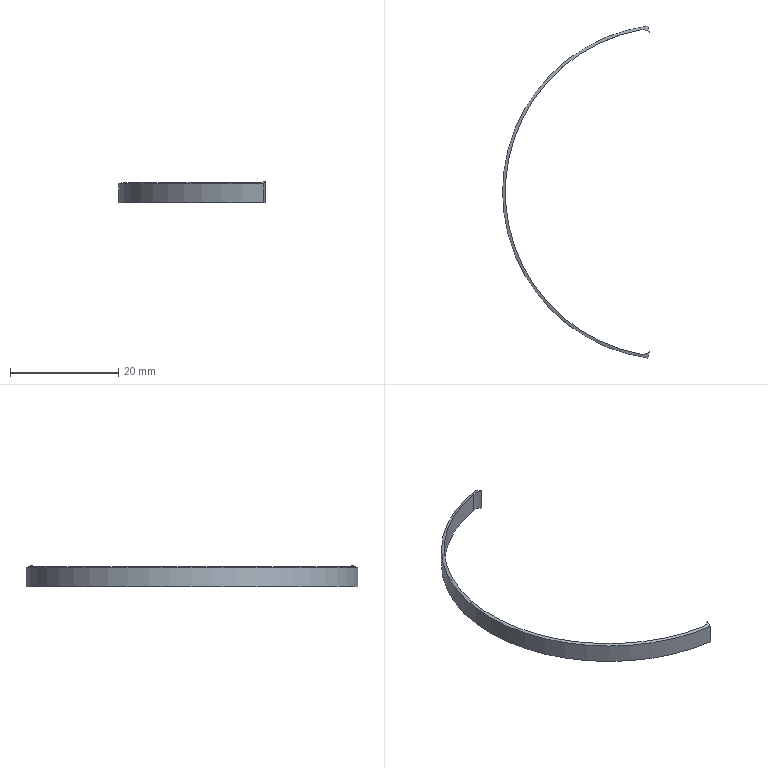Part | STEP file | 1 solid | 8 faces | box 27.164 x 61.45 x 3.959 mm | volume 161.362 mm3 | cylinder 4 | plane 3 | cone 1 | commonest cylinder face diameters 4 x2 61 x1 62 x1
STEP:
#1=CARTESIAN_POINT('',(0.,0.,0.));
#2=DIRECTION('',(0.,0.,1.));
#3=DIRECTION('',(1.,0.,0.));
#4=AXIS2_PLACEMENT_3D('',#1,#2,#3);
#5=CARTESIAN_POINT('',(26.179,127.81,-5.45));
#6=VERTEX_POINT('',#5);
#7=CARTESIAN_POINT('',(26.179,187.831,-5.45));
#8=VERTEX_POINT('',#7);
#9=CARTESIAN_POINT('',(31.622,157.82,-5.45));
#10=DIRECTION('',(0.,0.,-1.));
#11=DIRECTION('',(1.,0.,0.));
#12=AXIS2_PLACEMENT_3D('',#9,#10,#11);
#13=CIRCLE('',#12,30.5);
#14=CARTESIAN_POINT('',(31.622,157.82,-15.65));
#15=DIRECTION('',(0.,0.,1.));
#16=DIRECTION('',(1.,0.,0.));
#17=AXIS2_PLACEMENT_3D('',#14,#15,#16);
#18=CYLINDRICAL_SURFACE('',#17,30.5);
#19=CARTESIAN_POINT('',(6.283,10.2));
#20=DIRECTION('',(-1.,0.));
#21=VECTOR('',#20,1.);
#22=LINE('',#19,#21);
#23=(GEOMETRIC_REPRESENTATION_CONTEXT(2)PARAMETRIC_REPRESENTATION_CONTEXT()REPRESENTATION_CONTEXT('',''));
#24=DEFINITIONAL_REPRESENTATION('',(#22),#23);
#25=PCURVE('',#18,#24);
#26=CARTESIAN_POINT('',(31.622,157.82,-5.65));
#27=DIRECTION('',(0.,0.,-1.));
#28=DIRECTION('',(-1.,0.,0.));
#29=AXIS2_PLACEMENT_3D('',#26,#27,#28);
#30=CONICAL_SURFACE('',#29,31.,1.19);
#31=CARTESIAN_POINT('',(3.142,-0.2));
#32=DIRECTION('',(1.,0.));
#33=VECTOR('',#32,1.);
#34=LINE('',#31,#33);
#35=(GEOMETRIC_REPRESENTATION_CONTEXT(2)PARAMETRIC_REPRESENTATION_CONTEXT()REPRESENTATION_CONTEXT('',''));
#36=DEFINITIONAL_REPRESENTATION('',(#34),#35);
#37=PCURVE('',#30,#36);
#38=SURFACE_CURVE('',#13,(#25,#37),.PCURVE_S1.);
#39=EDGE_CURVE('',#6,#8,#38,.T.);
#40=ORIENTED_EDGE('',*,*,#39,.T.);
#41=CARTESIAN_POINT('',(26.179,187.831,-9.15));
#42=VERTEX_POINT('',#41);
#43=CARTESIAN_POINT('',(26.179,187.831,-15.65));
#44=DIRECTION('',(0.,0.,-1.));
#45=VECTOR('',#44,1.);
#46=LINE('',#43,#45);
#47=CARTESIAN_POINT('',(1.75,0.));
#48=DIRECTION('',(0.,-1.));
#49=VECTOR('',#48,1.);
#50=LINE('',#47,#49);
#51=(GEOMETRIC_REPRESENTATION_CONTEXT(2)PARAMETRIC_REPRESENTATION_CONTEXT()REPRESENTATION_CONTEXT('',''));
#52=DEFINITIONAL_REPRESENTATION('',(#50),#51);
#53=PCURVE('',#18,#52);
#54=CARTESIAN_POINT('',(26.536,185.863,-15.65));
#55=DIRECTION('',(0.,0.,-1.));
#56=DIRECTION('',(-1.,0.,0.));
#57=AXIS2_PLACEMENT_3D('',#54,#55,#56);
#58=CYLINDRICAL_SURFACE('',#57,2.);
#59=CARTESIAN_POINT('',(1.391,0.));
#60=DIRECTION('',(0.,1.));
#61=VECTOR('',#60,1.);
#62=LINE('',#59,#61);
#63=(GEOMETRIC_REPRESENTATION_CONTEXT(2)PARAMETRIC_REPRESENTATION_CONTEXT()REPRESENTATION_CONTEXT('',''));
#64=DEFINITIONAL_REPRESENTATION('',(#62),#63);
#65=PCURVE('',#58,#64);
#66=SURFACE_CURVE('',#46,(#53,#65),.PCURVE_S1.);
#67=EDGE_CURVE('',#8,#42,#66,.T.);
#68=ORIENTED_EDGE('',*,*,#67,.T.);
#69=CARTESIAN_POINT('',(26.179,127.81,-9.15));
#70=VERTEX_POINT('',#69);
#71=CARTESIAN_POINT('',(31.622,157.82,-9.15));
#72=DIRECTION('',(0.,0.,1.));
#73=DIRECTION('',(1.,0.,0.));
#74=AXIS2_PLACEMENT_3D('',#71,#72,#73);
#75=CIRCLE('',#74,30.5);
#76=CARTESIAN_POINT('',(0.,6.5));
#77=DIRECTION('',(1.,0.));
#78=VECTOR('',#77,1.);
#79=LINE('',#76,#78);
#80=(GEOMETRIC_REPRESENTATION_CONTEXT(2)PARAMETRIC_REPRESENTATION_CONTEXT()REPRESENTATION_CONTEXT('',''));
#81=DEFINITIONAL_REPRESENTATION('',(#79),#80);
#82=PCURVE('',#18,#81);
#83=CARTESIAN_POINT('',(65.122,157.82,-9.15));
#84=DIRECTION('',(0.,0.,1.));
#85=DIRECTION('',(1.,0.,0.));
#86=AXIS2_PLACEMENT_3D('',#83,#84,#85);
#87=PLANE('',#86);
#88=CARTESIAN_POINT('',(-33.5,0.));
#89=DIRECTION('',(1.,0.));
#90=AXIS2_PLACEMENT_2D('',#88,#89);
#91=CIRCLE('',#90,30.5);
#92=(GEOMETRIC_REPRESENTATION_CONTEXT(2)PARAMETRIC_REPRESENTATION_CONTEXT()REPRESENTATION_CONTEXT('',''));
#93=DEFINITIONAL_REPRESENTATION('',(#91),#92);
#94=PCURVE('',#87,#93);
#95=SURFACE_CURVE('',#75,(#82,#94),.PCURVE_S1.);
#96=EDGE_CURVE('',#42,#70,#95,.T.);
#97=ORIENTED_EDGE('',*,*,#96,.T.);
#98=CARTESIAN_POINT('',(26.179,127.81,-15.65));
#99=DIRECTION('',(0.,0.,1.));
#100=VECTOR('',#99,1.);
#101=LINE('',#98,#100);
#102=CARTESIAN_POINT('',(4.533,0.));
#103=DIRECTION('',(0.,1.));
#104=VECTOR('',#103,1.);
#105=LINE('',#102,#104);
#106=(GEOMETRIC_REPRESENTATION_CONTEXT(2)PARAMETRIC_REPRESENTATION_CONTEXT()REPRESENTATION_CONTEXT('',''));
#107=DEFINITIONAL_REPRESENTATION('',(#105),#106);
#108=PCURVE('',#18,#107);
#109=CARTESIAN_POINT('',(26.536,129.778,-15.65));
#110=DIRECTION('',(0.,0.,1.));
#111=DIRECTION('',(1.,0.,0.));
#112=AXIS2_PLACEMENT_3D('',#109,#110,#111);
#113=CYLINDRICAL_SURFACE('',#112,2.);
#114=CARTESIAN_POINT('',(4.533,0.));
#115=DIRECTION('',(0.,1.));
#116=VECTOR('',#115,1.);
#117=LINE('',#114,#116);
#118=(GEOMETRIC_REPRESENTATION_CONTEXT(2)PARAMETRIC_REPRESENTATION_CONTEXT()REPRESENTATION_CONTEXT('',''));
#119=DEFINITIONAL_REPRESENTATION('',(#117),#118);
#120=PCURVE('',#113,#119);
#121=SURFACE_CURVE('',#101,(#108,#120),.PCURVE_S1.);
#122=EDGE_CURVE('',#70,#6,#121,.T.);
#123=ORIENTED_EDGE('',*,*,#122,.T.);
#124=EDGE_LOOP('',(#40,#68,#97,#123));
#125=FACE_BOUND('',#124,.F.);
#126=ADVANCED_FACE('',(#125),#18,.F.);
#127=CARTESIAN_POINT('',(27.501,127.095,-5.65));
#128=VERTEX_POINT('',#127);
#129=CARTESIAN_POINT('',(27.786,128.216,-5.191));
#130=VERTEX_POINT('',#129);
#131=CARTESIAN_POINT('',(27.501,127.095,-5.65));
#132=CARTESIAN_POINT('',(27.596,127.469,-5.497));
#133=CARTESIAN_POINT('',(27.691,127.843,-5.344));
#134=CARTESIAN_POINT('',(27.786,128.216,-5.191));
#135=B_SPLINE_CURVE_WITH_KNOTS('',3,(#131,#132,#133,#134),.UNSPECIFIED.,.F.,.F.,(4,4),(0.,0.001245),.PIECEWISE_BEZIER_KNOTS.);
#136=CARTESIAN_POINT('',(4.846,-0.000000009));
#137=CARTESIAN_POINT('',(4.846,-0.006962));
#138=CARTESIAN_POINT('',(4.846,-0.02089));
#139=CARTESIAN_POINT('',(4.845,-0.04177));
#140=CARTESIAN_POINT('',(4.845,-0.06266));
#141=CARTESIAN_POINT('',(4.845,-0.08354));
#142=CARTESIAN_POINT('',(4.845,-0.1044));
#143=CARTESIAN_POINT('',(4.845,-0.1253));
#144=CARTESIAN_POINT('',(4.844,-0.1462));
#145=CARTESIAN_POINT('',(4.844,-0.1671));
#146=CARTESIAN_POINT('',(4.844,-0.188));
#147=CARTESIAN_POINT('',(4.844,-0.2088));
#148=CARTESIAN_POINT('',(4.844,-0.2297));
#149=CARTESIAN_POINT('',(4.843,-0.2506));
#150=CARTESIAN_POINT('',(4.843,-0.2715));
#151=CARTESIAN_POINT('',(4.843,-0.2924));
#152=CARTESIAN_POINT('',(4.843,-0.3133));
#153=CARTESIAN_POINT('',(4.843,-0.3341));
#154=CARTESIAN_POINT('',(4.842,-0.355));
#155=CARTESIAN_POINT('',(4.842,-0.3759));
#156=CARTESIAN_POINT('',(4.842,-0.3968));
#157=CARTESIAN_POINT('',(4.842,-0.4177));
#158=CARTESIAN_POINT('',(4.841,-0.4385));
#159=CARTESIAN_POINT('',(4.841,-0.4525));
#160=CARTESIAN_POINT('',(4.841,-0.4594));
#161=B_SPLINE_CURVE_WITH_KNOTS('',3,(#136,#137,#138,#139,#140,#141,#142,#143,#144,#145,#146,#147,#148,#149,#150,#151,#152,#153,#154,#155,#156,#157,#158,#159,#160),.UNSPECIFIED.,.F.,.F.,(4,1,1,1,1,1,1,1,1,1,1,1,1,1,1,1,1,1,1,1,1,1,4),(0.,0.00005657,0.0001131,0.0001697,0.0002263,0.0002828,0.0003394,0.000396,0.0004525,0.0005091,0.0005657,0.0006223,0.0006788,0.0007354,0.000792,0.0008485,0.0009051,0.0009617,0.001018,0.001075,0.001131,0.001188,0.001245),.QUASI_UNIFORM_KNOTS.);
#162=(GEOMETRIC_REPRESENTATION_CONTEXT(2)PARAMETRIC_REPRESENTATION_CONTEXT()REPRESENTATION_CONTEXT('',''));
#163=DEFINITIONAL_REPRESENTATION('',(#161),#162);
#164=PCURVE('',#30,#163);
#165=CARTESIAN_POINT('',(27.372,126.591,-10.65));
#166=DIRECTION('',(-0.9691,0.2469,0.));
#167=DIRECTION('',(-0.2469,-0.9691,0.));
#168=AXIS2_PLACEMENT_3D('',#165,#166,#167);
#169=PLANE('',#168);
#170=CARTESIAN_POINT('',(-0.5206,5.));
#171=CARTESIAN_POINT('',(-0.9062,5.153));
#172=CARTESIAN_POINT('',(-1.292,5.306));
#173=CARTESIAN_POINT('',(-1.677,5.459));
#174=B_SPLINE_CURVE_WITH_KNOTS('',3,(#170,#171,#172,#173),.UNSPECIFIED.,.F.,.F.,(4,4),(0.,0.001245),.PIECEWISE_BEZIER_KNOTS.);
#175=(GEOMETRIC_REPRESENTATION_CONTEXT(2)PARAMETRIC_REPRESENTATION_CONTEXT()REPRESENTATION_CONTEXT('',''));
#176=DEFINITIONAL_REPRESENTATION('',(#174),#175);
#177=PCURVE('',#169,#176);
#178=SURFACE_CURVE('',#135,(#164,#177),.PCURVE_S1.);
#179=EDGE_CURVE('',#128,#130,#178,.T.);
#180=ORIENTED_EDGE('',*,*,#179,.T.);
#181=CARTESIAN_POINT('',(27.786,128.216,-5.191));
#182=CARTESIAN_POINT('',(27.567,128.041,-5.271));
#183=CARTESIAN_POINT('',(27.311,127.912,-5.337));
#184=CARTESIAN_POINT('',(26.896,127.805,-5.404));
#185=CARTESIAN_POINT('',(26.752,127.784,-5.421));
#186=CARTESIAN_POINT('',(26.466,127.774,-5.444));
#187=CARTESIAN_POINT('',(26.323,127.784,-5.45));
#188=CARTESIAN_POINT('',(26.179,127.81,-5.45));
#189=B_SPLINE_CURVE_WITH_KNOTS('',3,(#181,#182,#183,#184,#185,#186,#187,#188),.UNSPECIFIED.,.F.,.F.,(4,2,2,4),(-0.000354,0.0005088,0.0009403,0.001372),.UNSPECIFIED.);
#190=CARTESIAN_POINT('',(4.841,-0.4594));
#191=CARTESIAN_POINT('',(4.842,-0.4521));
#192=CARTESIAN_POINT('',(4.843,-0.4377));
#193=CARTESIAN_POINT('',(4.845,-0.4168));
#194=CARTESIAN_POINT('',(4.847,-0.3968));
#195=CARTESIAN_POINT('',(4.849,-0.3776));
#196=CARTESIAN_POINT('',(4.851,-0.3592));
#197=CARTESIAN_POINT('',(4.853,-0.3418));
#198=CARTESIAN_POINT('',(4.855,-0.3252));
#199=CARTESIAN_POINT('',(4.857,-0.3095));
#200=CARTESIAN_POINT('',(4.86,-0.2948));
#201=CARTESIAN_POINT('',(4.862,-0.2811));
#202=CARTESIAN_POINT('',(4.864,-0.2684));
#203=CARTESIAN_POINT('',(4.867,-0.2567));
#204=CARTESIAN_POINT('',(4.869,-0.246));
#205=CARTESIAN_POINT('',(4.872,-0.2364));
#206=CARTESIAN_POINT('',(4.874,-0.2278));
#207=CARTESIAN_POINT('',(4.876,-0.2204));
#208=CARTESIAN_POINT('',(4.879,-0.2142));
#209=CARTESIAN_POINT('',(4.882,-0.209));
#210=CARTESIAN_POINT('',(4.884,-0.205));
#211=CARTESIAN_POINT('',(4.887,-0.2021));
#212=CARTESIAN_POINT('',(4.889,-0.2004));
#213=CARTESIAN_POINT('',(4.891,-0.2));
#214=CARTESIAN_POINT('',(4.892,-0.2));
#215=B_SPLINE_CURVE_WITH_KNOTS('',3,(#190,#191,#192,#193,#194,#195,#196,#197,#198,#199,#200,#201,#202,#203,#204,#205,#206,#207,#208,#209,#210,#211,#212,#213,#214),.UNSPECIFIED.,.F.,.F.,(4,1,1,1,1,1,1,1,1,1,1,1,1,1,1,1,1,1,1,1,1,1,4),(-0.000354,-0.0002756,-0.0001971,-0.0001187,-0.00004026,0.00003818,0.0001166,0.0001951,0.0002735,0.0003519,0.0004304,0.0005088,0.0005873,0.0006657,0.0007442,0.0008226,0.000901,0.0009795,0.001058,0.001136,0.001215,0.001293,0.001372),.UNSPECIFIED.);
#216=(GEOMETRIC_REPRESENTATION_CONTEXT(2)PARAMETRIC_REPRESENTATION_CONTEXT()REPRESENTATION_CONTEXT('',''));
#217=DEFINITIONAL_REPRESENTATION('',(#215),#216);
#218=PCURVE('',#30,#217);
#219=CARTESIAN_POINT('',(5.387,10.459));
#220=CARTESIAN_POINT('',(5.375,10.452));
#221=CARTESIAN_POINT('',(5.349,10.438));
#222=CARTESIAN_POINT('',(5.311,10.417));
#223=CARTESIAN_POINT('',(5.273,10.397));
#224=CARTESIAN_POINT('',(5.234,10.378));
#225=CARTESIAN_POINT('',(5.196,10.359));
#226=CARTESIAN_POINT('',(5.157,10.342));
#227=CARTESIAN_POINT('',(5.119,10.325));
#228=CARTESIAN_POINT('',(5.08,10.31));
#229=CARTESIAN_POINT('',(5.042,10.295));
#230=CARTESIAN_POINT('',(5.003,10.281));
#231=CARTESIAN_POINT('',(4.964,10.268));
#232=CARTESIAN_POINT('',(4.925,10.257));
#233=CARTESIAN_POINT('',(4.886,10.246));
#234=CARTESIAN_POINT('',(4.847,10.236));
#235=CARTESIAN_POINT('',(4.807,10.228));
#236=CARTESIAN_POINT('',(4.768,10.22));
#237=CARTESIAN_POINT('',(4.729,10.214));
#238=CARTESIAN_POINT('',(4.69,10.209));
#239=CARTESIAN_POINT('',(4.651,10.205));
#240=CARTESIAN_POINT('',(4.612,10.202));
#241=CARTESIAN_POINT('',(4.573,10.2));
#242=CARTESIAN_POINT('',(4.546,10.2));
#243=CARTESIAN_POINT('',(4.533,10.2));
#244=B_SPLINE_CURVE_WITH_KNOTS('',3,(#219,#220,#221,#222,#223,#224,#225,#226,#227,#228,#229,#230,#231,#232,#233,#234,#235,#236,#237,#238,#239,#240,#241,#242,#243),.UNSPECIFIED.,.F.,.F.,(4,1,1,1,1,1,1,1,1,1,1,1,1,1,1,1,1,1,1,1,1,1,4),(-0.000354,-0.0002756,-0.0001971,-0.0001187,-0.00004026,0.00003818,0.0001166,0.0001951,0.0002735,0.0003519,0.0004304,0.0005088,0.0005873,0.0006657,0.0007442,0.0008226,0.000901,0.0009795,0.001058,0.001136,0.001215,0.001293,0.001372),.UNSPECIFIED.);
#245=(GEOMETRIC_REPRESENTATION_CONTEXT(2)PARAMETRIC_REPRESENTATION_CONTEXT()REPRESENTATION_CONTEXT('',''));
#246=DEFINITIONAL_REPRESENTATION('',(#244),#245);
#247=PCURVE('',#113,#246);
#248=SURFACE_CURVE('',#189,(#218,#247),.PCURVE_S1.);
#249=EDGE_CURVE('',#130,#6,#248,.T.);
#250=ORIENTED_EDGE('',*,*,#249,.T.);
#251=ORIENTED_EDGE('',*,*,#39,.T.);
#252=CARTESIAN_POINT('',(27.786,187.424,-5.191));
#253=VERTEX_POINT('',#252);
#254=CARTESIAN_POINT('',(26.179,187.831,-5.45));
#255=CARTESIAN_POINT('',(26.323,187.857,-5.45));
#256=CARTESIAN_POINT('',(26.466,187.867,-5.444));
#257=CARTESIAN_POINT('',(26.752,187.856,-5.421));
#258=CARTESIAN_POINT('',(26.897,187.835,-5.404));
#259=CARTESIAN_POINT('',(27.31,187.729,-5.337));
#260=CARTESIAN_POINT('',(27.568,187.599,-5.271));
#261=CARTESIAN_POINT('',(27.786,187.424,-5.191));
#262=B_SPLINE_CURVE_WITH_KNOTS('',3,(#254,#255,#256,#257,#258,#259,#260,#261),.UNSPECIFIED.,.F.,.F.,(4,2,2,4),(0.,0.0004306,0.0008612,0.001722),.UNSPECIFIED.);
#263=CARTESIAN_POINT('',(7.675,-0.2));
#264=CARTESIAN_POINT('',(7.675,-0.2));
#265=CARTESIAN_POINT('',(7.677,-0.2004));
#266=CARTESIAN_POINT('',(7.68,-0.2021));
#267=CARTESIAN_POINT('',(7.682,-0.205));
#268=CARTESIAN_POINT('',(7.685,-0.209));
#269=CARTESIAN_POINT('',(7.687,-0.2142));
#270=CARTESIAN_POINT('',(7.69,-0.2205));
#271=CARTESIAN_POINT('',(7.692,-0.2279));
#272=CARTESIAN_POINT('',(7.695,-0.2364));
#273=CARTESIAN_POINT('',(7.697,-0.2461));
#274=CARTESIAN_POINT('',(7.7,-0.2568));
#275=CARTESIAN_POINT('',(7.702,-0.2684));
#276=CARTESIAN_POINT('',(7.704,-0.2811));
#277=CARTESIAN_POINT('',(7.707,-0.2948));
#278=CARTESIAN_POINT('',(7.709,-0.3095));
#279=CARTESIAN_POINT('',(7.711,-0.3252));
#280=CARTESIAN_POINT('',(7.713,-0.3418));
#281=CARTESIAN_POINT('',(7.715,-0.3592));
#282=CARTESIAN_POINT('',(7.718,-0.3776));
#283=CARTESIAN_POINT('',(7.72,-0.3968));
#284=CARTESIAN_POINT('',(7.721,-0.4169));
#285=CARTESIAN_POINT('',(7.723,-0.4377));
#286=CARTESIAN_POINT('',(7.725,-0.4521));
#287=CARTESIAN_POINT('',(7.725,-0.4594));
#288=B_SPLINE_CURVE_WITH_KNOTS('',3,(#263,#264,#265,#266,#267,#268,#269,#270,#271,#272,#273,#274,#275,#276,#277,#278,#279,#280,#281,#282,#283,#284,#285,#286,#287),.UNSPECIFIED.,.F.,.F.,(4,1,1,1,1,1,1,1,1,1,1,1,1,1,1,1,1,1,1,1,1,1,4),(0.,0.00007829,0.0001566,0.0002349,0.0003132,0.0003915,0.0004697,0.000548,0.0006263,0.0007046,0.0007829,0.0008612,0.0009395,0.001018,0.001096,0.001174,0.001253,0.001331,0.001409,0.001488,0.001566,0.001644,0.001722),.QUASI_UNIFORM_KNOTS.);
#289=(GEOMETRIC_REPRESENTATION_CONTEXT(2)PARAMETRIC_REPRESENTATION_CONTEXT()REPRESENTATION_CONTEXT('',''));
#290=DEFINITIONAL_REPRESENTATION('',(#288),#289);
#291=PCURVE('',#30,#290);
#292=CARTESIAN_POINT('',(1.391,-10.2));
#293=CARTESIAN_POINT('',(1.405,-10.2));
#294=CARTESIAN_POINT('',(1.431,-10.2));
#295=CARTESIAN_POINT('',(1.47,-10.202));
#296=CARTESIAN_POINT('',(1.51,-10.205));
#297=CARTESIAN_POINT('',(1.549,-10.209));
#298=CARTESIAN_POINT('',(1.588,-10.214));
#299=CARTESIAN_POINT('',(1.627,-10.22));
#300=CARTESIAN_POINT('',(1.666,-10.228));
#301=CARTESIAN_POINT('',(1.705,-10.236));
#302=CARTESIAN_POINT('',(1.745,-10.246));
#303=CARTESIAN_POINT('',(1.784,-10.257));
#304=CARTESIAN_POINT('',(1.823,-10.268));
#305=CARTESIAN_POINT('',(1.861,-10.281));
#306=CARTESIAN_POINT('',(1.9,-10.295));
#307=CARTESIAN_POINT('',(1.939,-10.31));
#308=CARTESIAN_POINT('',(1.977,-10.325));
#309=CARTESIAN_POINT('',(2.016,-10.342));
#310=CARTESIAN_POINT('',(2.054,-10.359));
#311=CARTESIAN_POINT('',(2.093,-10.378));
#312=CARTESIAN_POINT('',(2.131,-10.397));
#313=CARTESIAN_POINT('',(2.169,-10.417));
#314=CARTESIAN_POINT('',(2.208,-10.438));
#315=CARTESIAN_POINT('',(2.233,-10.452));
#316=CARTESIAN_POINT('',(2.246,-10.459));
#317=B_SPLINE_CURVE_WITH_KNOTS('',3,(#292,#293,#294,#295,#296,#297,#298,#299,#300,#301,#302,#303,#304,#305,#306,#307,#308,#309,#310,#311,#312,#313,#314,#315,#316),.UNSPECIFIED.,.F.,.F.,(4,1,1,1,1,1,1,1,1,1,1,1,1,1,1,1,1,1,1,1,1,1,4),(0.,0.00007829,0.0001566,0.0002349,0.0003132,0.0003915,0.0004697,0.000548,0.0006263,0.0007046,0.0007829,0.0008612,0.0009395,0.001018,0.001096,0.001174,0.001253,0.001331,0.001409,0.001488,0.001566,0.001644,0.001722),.QUASI_UNIFORM_KNOTS.);
#318=(GEOMETRIC_REPRESENTATION_CONTEXT(2)PARAMETRIC_REPRESENTATION_CONTEXT()REPRESENTATION_CONTEXT('',''));
#319=DEFINITIONAL_REPRESENTATION('',(#317),#318);
#320=PCURVE('',#58,#319);
#321=SURFACE_CURVE('',#262,(#291,#320),.PCURVE_S1.);
#322=EDGE_CURVE('',#8,#253,#321,.T.);
#323=ORIENTED_EDGE('',*,*,#322,.T.);
#324=CARTESIAN_POINT('',(27.501,188.545,-5.65));
#325=VERTEX_POINT('',#324);
#326=CARTESIAN_POINT('',(27.786,187.424,-5.191));
#327=CARTESIAN_POINT('',(27.691,187.798,-5.344));
#328=CARTESIAN_POINT('',(27.596,188.171,-5.497));
#329=CARTESIAN_POINT('',(27.501,188.545,-5.65));
#330=B_SPLINE_CURVE_WITH_KNOTS('',3,(#326,#327,#328,#329),.UNSPECIFIED.,.F.,.F.,(4,4),(0.,0.001245),.PIECEWISE_BEZIER_KNOTS.);
#331=CARTESIAN_POINT('',(7.725,-0.4594));
#332=CARTESIAN_POINT('',(7.725,-0.4525));
#333=CARTESIAN_POINT('',(7.725,-0.4385));
#334=CARTESIAN_POINT('',(7.725,-0.4177));
#335=CARTESIAN_POINT('',(7.724,-0.3968));
#336=CARTESIAN_POINT('',(7.724,-0.3759));
#337=CARTESIAN_POINT('',(7.724,-0.355));
#338=CARTESIAN_POINT('',(7.724,-0.3341));
#339=CARTESIAN_POINT('',(7.724,-0.3133));
#340=CARTESIAN_POINT('',(7.723,-0.2924));
#341=CARTESIAN_POINT('',(7.723,-0.2715));
#342=CARTESIAN_POINT('',(7.723,-0.2506));
#343=CARTESIAN_POINT('',(7.723,-0.2297));
#344=CARTESIAN_POINT('',(7.723,-0.2088));
#345=CARTESIAN_POINT('',(7.722,-0.188));
#346=CARTESIAN_POINT('',(7.722,-0.1671));
#347=CARTESIAN_POINT('',(7.722,-0.1462));
#348=CARTESIAN_POINT('',(7.722,-0.1253));
#349=CARTESIAN_POINT('',(7.722,-0.1044));
#350=CARTESIAN_POINT('',(7.721,-0.08354));
#351=CARTESIAN_POINT('',(7.721,-0.06266));
#352=CARTESIAN_POINT('',(7.721,-0.04177));
#353=CARTESIAN_POINT('',(7.721,-0.02089));
#354=CARTESIAN_POINT('',(7.721,-0.006962));
#355=CARTESIAN_POINT('',(7.721,0.000000003));
#356=B_SPLINE_CURVE_WITH_KNOTS('',3,(#331,#332,#333,#334,#335,#336,#337,#338,#339,#340,#341,#342,#343,#344,#345,#346,#347,#348,#349,#350,#351,#352,#353,#354,#355),.UNSPECIFIED.,.F.,.F.,(4,1,1,1,1,1,1,1,1,1,1,1,1,1,1,1,1,1,1,1,1,1,4),(0.,0.00005657,0.0001131,0.0001697,0.0002263,0.0002828,0.0003394,0.000396,0.0004525,0.0005091,0.0005657,0.0006223,0.0006788,0.0007354,0.000792,0.0008485,0.0009051,0.0009617,0.001018,0.001075,0.001131,0.001188,0.001245),.QUASI_UNIFORM_KNOTS.);
#357=(GEOMETRIC_REPRESENTATION_CONTEXT(2)PARAMETRIC_REPRESENTATION_CONTEXT()REPRESENTATION_CONTEXT('',''));
#358=DEFINITIONAL_REPRESENTATION('',(#356),#357);
#359=PCURVE('',#30,#358);
#360=CARTESIAN_POINT('',(28.322,185.32,-10.65));
#361=DIRECTION('',(-0.9691,-0.2469,0.));
#362=DIRECTION('',(0.2469,-0.9691,0.));
#363=AXIS2_PLACEMENT_3D('',#360,#361,#362);
#364=PLANE('',#363);
#365=CARTESIAN_POINT('',(-2.171,5.459));
#366=CARTESIAN_POINT('',(-2.557,5.306));
#367=CARTESIAN_POINT('',(-2.942,5.153));
#368=CARTESIAN_POINT('',(-3.328,5.));
#369=B_SPLINE_CURVE_WITH_KNOTS('',3,(#365,#366,#367,#368),.UNSPECIFIED.,.F.,.F.,(4,4),(0.,0.001245),.PIECEWISE_BEZIER_KNOTS.);
#370=(GEOMETRIC_REPRESENTATION_CONTEXT(2)PARAMETRIC_REPRESENTATION_CONTEXT()REPRESENTATION_CONTEXT('',''));
#371=DEFINITIONAL_REPRESENTATION('',(#369),#370);
#372=PCURVE('',#364,#371);
#373=SURFACE_CURVE('',#330,(#359,#372),.PCURVE_S1.);
#374=EDGE_CURVE('',#253,#325,#373,.T.);
#375=ORIENTED_EDGE('',*,*,#374,.T.);
#376=CARTESIAN_POINT('',(31.622,157.82,-5.65));
#377=DIRECTION('',(0.,0.,1.));
#378=DIRECTION('',(-0.809,0.5878,0.));
#379=AXIS2_PLACEMENT_3D('',#376,#377,#378);
#380=CIRCLE('',#379,31.);
#381=CARTESIAN_POINT('',(13.195,-0.000000038));
#382=DIRECTION('',(-1.,0.));
#383=VECTOR('',#382,1.);
#384=LINE('',#381,#383);
#385=(GEOMETRIC_REPRESENTATION_CONTEXT(2)PARAMETRIC_REPRESENTATION_CONTEXT()REPRESENTATION_CONTEXT('',''));
#386=DEFINITIONAL_REPRESENTATION('',(#384),#385);
#387=PCURVE('',#30,#386);
#388=CARTESIAN_POINT('',(31.622,157.82,-7.4));
#389=DIRECTION('',(0.,0.,-1.));
#390=DIRECTION('',(-1.,0.,0.));
#391=AXIS2_PLACEMENT_3D('',#388,#389,#390);
#392=CYLINDRICAL_SURFACE('',#391,31.);
#393=CARTESIAN_POINT('',(6.912,-1.75));
#394=DIRECTION('',(-1.,0.));
#395=VECTOR('',#394,1.);
#396=LINE('',#393,#395);
#397=(GEOMETRIC_REPRESENTATION_CONTEXT(2)PARAMETRIC_REPRESENTATION_CONTEXT()REPRESENTATION_CONTEXT('',''));
#398=DEFINITIONAL_REPRESENTATION('',(#396),#397);
#399=PCURVE('',#392,#398);
#400=SURFACE_CURVE('',#380,(#387,#399),.PCURVE_S1.);
#401=EDGE_CURVE('',#325,#128,#400,.T.);
#402=ORIENTED_EDGE('',*,*,#401,.T.);
#403=EDGE_LOOP('',(#180,#250,#251,#323,#375,#402));
#404=FACE_BOUND('',#403,.T.);
#405=ADVANCED_FACE('',(#404),#30,.T.);
#406=CARTESIAN_POINT('',(27.786,128.216,-9.15));
#407=VERTEX_POINT('',#406);
#408=CARTESIAN_POINT('',(27.786,128.216,-15.65));
#409=DIRECTION('',(0.,0.,1.));
#410=VECTOR('',#409,1.);
#411=LINE('',#408,#410);
#412=CARTESIAN_POINT('',(5.387,0.));
#413=DIRECTION('',(0.,1.));
#414=VECTOR('',#413,1.);
#415=LINE('',#412,#414);
#416=(GEOMETRIC_REPRESENTATION_CONTEXT(2)PARAMETRIC_REPRESENTATION_CONTEXT()REPRESENTATION_CONTEXT('',''));
#417=DEFINITIONAL_REPRESENTATION('',(#415),#416);
#418=PCURVE('',#113,#417);
#419=CARTESIAN_POINT('',(-1.677,-5.));
#420=DIRECTION('',(0.,1.));
#421=VECTOR('',#420,1.);
#422=LINE('',#419,#421);
#423=(GEOMETRIC_REPRESENTATION_CONTEXT(2)PARAMETRIC_REPRESENTATION_CONTEXT()REPRESENTATION_CONTEXT('',''));
#424=DEFINITIONAL_REPRESENTATION('',(#422),#423);
#425=PCURVE('',#169,#424);
#426=SURFACE_CURVE('',#411,(#418,#425),.PCURVE_S1.);
#427=EDGE_CURVE('',#407,#130,#426,.T.);
#428=ORIENTED_EDGE('',*,*,#427,.T.);
#429=ORIENTED_EDGE('',*,*,#249,.T.);
#430=ORIENTED_EDGE('',*,*,#122,.F.);
#431=CARTESIAN_POINT('',(26.536,129.778,-9.15));
#432=DIRECTION('',(0.,0.,1.));
#433=DIRECTION('',(1.,0.,0.));
#434=AXIS2_PLACEMENT_3D('',#431,#432,#433);
#435=CIRCLE('',#434,2.);
#436=CARTESIAN_POINT('',(0.,6.5));
#437=DIRECTION('',(1.,0.));
#438=VECTOR('',#437,1.);
#439=LINE('',#436,#438);
#440=(GEOMETRIC_REPRESENTATION_CONTEXT(2)PARAMETRIC_REPRESENTATION_CONTEXT()REPRESENTATION_CONTEXT('',''));
#441=DEFINITIONAL_REPRESENTATION('',(#439),#440);
#442=PCURVE('',#113,#441);
#443=CARTESIAN_POINT('',(-38.586,-28.043));
#444=DIRECTION('',(1.,0.));
#445=AXIS2_PLACEMENT_2D('',#443,#444);
#446=CIRCLE('',#445,2.);
#447=(GEOMETRIC_REPRESENTATION_CONTEXT(2)PARAMETRIC_REPRESENTATION_CONTEXT()REPRESENTATION_CONTEXT('',''));
#448=DEFINITIONAL_REPRESENTATION('',(#446),#447);
#449=PCURVE('',#87,#448);
#450=SURFACE_CURVE('',#435,(#442,#449),.PCURVE_S1.);
#451=EDGE_CURVE('',#70,#407,#450,.T.);
#452=ORIENTED_EDGE('',*,*,#451,.T.);
#453=EDGE_LOOP('',(#428,#429,#430,#452));
#454=FACE_BOUND('',#453,.F.);
#455=ADVANCED_FACE('',(#454),#113,.F.);
#456=CARTESIAN_POINT('',(27.501,188.545,-9.15));
#457=VERTEX_POINT('',#456);
#458=CARTESIAN_POINT('',(27.786,187.424,-9.15));
#459=VERTEX_POINT('',#458);
#460=CARTESIAN_POINT('',(28.322,185.32,-9.15));
#461=DIRECTION('',(0.2469,-0.9691,0.));
#462=VECTOR('',#461,1.);
#463=LINE('',#460,#462);
#464=CARTESIAN_POINT('',(-36.8,27.5));
#465=DIRECTION('',(0.2469,-0.9691));
#466=VECTOR('',#465,1.);
#467=LINE('',#464,#466);
#468=(GEOMETRIC_REPRESENTATION_CONTEXT(2)PARAMETRIC_REPRESENTATION_CONTEXT()REPRESENTATION_CONTEXT('',''));
#469=DEFINITIONAL_REPRESENTATION('',(#467),#468);
#470=PCURVE('',#87,#469);
#471=CARTESIAN_POINT('',(0.,1.5));
#472=DIRECTION('',(1.,0.));
#473=VECTOR('',#472,1.);
#474=LINE('',#471,#473);
#475=(GEOMETRIC_REPRESENTATION_CONTEXT(2)PARAMETRIC_REPRESENTATION_CONTEXT()REPRESENTATION_CONTEXT('',''));
#476=DEFINITIONAL_REPRESENTATION('',(#474),#475);
#477=PCURVE('',#364,#476);
#478=SURFACE_CURVE('',#463,(#470,#477),.PCURVE_S1.);
#479=EDGE_CURVE('',#457,#459,#478,.T.);
#480=ORIENTED_EDGE('',*,*,#479,.T.);
#481=CARTESIAN_POINT('',(26.536,185.863,-9.15));
#482=DIRECTION('',(0.,0.,-1.));
#483=DIRECTION('',(-1.,0.,0.));
#484=AXIS2_PLACEMENT_3D('',#481,#482,#483);
#485=CIRCLE('',#484,2.);
#486=CARTESIAN_POINT('',(-40.586,28.043));
#487=CARTESIAN_POINT('',(-40.586,31.507));
#488=CARTESIAN_POINT('',(-37.586,29.775));
#489=CARTESIAN_POINT('',(-34.586,28.043));
#490=CARTESIAN_POINT('',(-37.586,26.311));
#491=CARTESIAN_POINT('',(-40.586,24.578));
#492=CARTESIAN_POINT('',(-40.586,28.043));
#493=(BOUNDED_CURVE()B_SPLINE_CURVE(2,(#486,#487,#488,#489,#490,#491,#492),.UNSPECIFIED.,.T.,.F.)B_SPLINE_CURVE_WITH_KNOTS((1,2,2,2,2,1),(-2.094,0.,2.094,4.189,6.283,8.378),.UNSPECIFIED.)CURVE()GEOMETRIC_REPRESENTATION_ITEM()RATIONAL_B_SPLINE_CURVE((1.,0.5,1.,0.5,1.,0.5,1.))REPRESENTATION_ITEM(''));
#494=(GEOMETRIC_REPRESENTATION_CONTEXT(2)PARAMETRIC_REPRESENTATION_CONTEXT()REPRESENTATION_CONTEXT('',''));
#495=DEFINITIONAL_REPRESENTATION('',(#493),#494);
#496=PCURVE('',#87,#495);
#497=CARTESIAN_POINT('',(0.,-6.5));
#498=DIRECTION('',(1.,0.));
#499=VECTOR('',#498,1.);
#500=LINE('',#497,#499);
#501=(GEOMETRIC_REPRESENTATION_CONTEXT(2)PARAMETRIC_REPRESENTATION_CONTEXT()REPRESENTATION_CONTEXT('',''));
#502=DEFINITIONAL_REPRESENTATION('',(#500),#501);
#503=PCURVE('',#58,#502);
#504=SURFACE_CURVE('',#485,(#496,#503),.PCURVE_S1.);
#505=EDGE_CURVE('',#42,#459,#504,.T.);
#506=ORIENTED_EDGE('',*,*,#505,.F.);
#507=ORIENTED_EDGE('',*,*,#96,.T.);
#508=ORIENTED_EDGE('',*,*,#451,.T.);
#509=CARTESIAN_POINT('',(27.501,127.095,-9.15));
#510=VERTEX_POINT('',#509);
#511=CARTESIAN_POINT('',(27.372,126.591,-9.15));
#512=DIRECTION('',(-0.2469,-0.9691,0.));
#513=VECTOR('',#512,1.);
#514=LINE('',#511,#513);
#515=CARTESIAN_POINT('',(-37.75,-31.229));
#516=DIRECTION('',(-0.2469,-0.9691));
#517=VECTOR('',#516,1.);
#518=LINE('',#515,#517);
#519=(GEOMETRIC_REPRESENTATION_CONTEXT(2)PARAMETRIC_REPRESENTATION_CONTEXT()REPRESENTATION_CONTEXT('',''));
#520=DEFINITIONAL_REPRESENTATION('',(#518),#519);
#521=PCURVE('',#87,#520);
#522=CARTESIAN_POINT('',(0.,1.5));
#523=DIRECTION('',(1.,0.));
#524=VECTOR('',#523,1.);
#525=LINE('',#522,#524);
#526=(GEOMETRIC_REPRESENTATION_CONTEXT(2)PARAMETRIC_REPRESENTATION_CONTEXT()REPRESENTATION_CONTEXT('',''));
#527=DEFINITIONAL_REPRESENTATION('',(#525),#526);
#528=PCURVE('',#169,#527);
#529=SURFACE_CURVE('',#514,(#521,#528),.PCURVE_S1.);
#530=EDGE_CURVE('',#407,#510,#529,.T.);
#531=ORIENTED_EDGE('',*,*,#530,.T.);
#532=CARTESIAN_POINT('',(31.622,157.82,-9.15));
#533=DIRECTION('',(0.,0.,1.));
#534=DIRECTION('',(-1.,0.,0.));
#535=AXIS2_PLACEMENT_3D('',#532,#533,#534);
#536=CIRCLE('',#535,31.);
#537=CARTESIAN_POINT('',(-33.5,0.));
#538=DIRECTION('',(-1.,0.));
#539=AXIS2_PLACEMENT_2D('',#537,#538);
#540=CIRCLE('',#539,31.);
#541=(GEOMETRIC_REPRESENTATION_CONTEXT(2)PARAMETRIC_REPRESENTATION_CONTEXT()REPRESENTATION_CONTEXT('',''));
#542=DEFINITIONAL_REPRESENTATION('',(#540),#541);
#543=PCURVE('',#87,#542);
#544=CARTESIAN_POINT('',(6.283,1.75));
#545=DIRECTION('',(-1.,0.));
#546=VECTOR('',#545,1.);
#547=LINE('',#544,#546);
#548=(GEOMETRIC_REPRESENTATION_CONTEXT(2)PARAMETRIC_REPRESENTATION_CONTEXT()REPRESENTATION_CONTEXT('',''));
#549=DEFINITIONAL_REPRESENTATION('',(#547),#548);
#550=PCURVE('',#392,#549);
#551=SURFACE_CURVE('',#536,(#543,#550),.PCURVE_S1.);
#552=EDGE_CURVE('',#457,#510,#551,.T.);
#553=ORIENTED_EDGE('',*,*,#552,.F.);
#554=EDGE_LOOP('',(#480,#506,#507,#508,#531,#553));
#555=FACE_BOUND('',#554,.T.);
#556=ADVANCED_FACE('',(#555),#87,.F.);
#557=CARTESIAN_POINT('',(27.786,187.424,-15.65));
#558=DIRECTION('',(0.,0.,-1.));
#559=VECTOR('',#558,1.);
#560=LINE('',#557,#559);
#561=CARTESIAN_POINT('',(2.246,0.));
#562=DIRECTION('',(0.,1.));
#563=VECTOR('',#562,1.);
#564=LINE('',#561,#563);
#565=(GEOMETRIC_REPRESENTATION_CONTEXT(2)PARAMETRIC_REPRESENTATION_CONTEXT()REPRESENTATION_CONTEXT('',''));
#566=DEFINITIONAL_REPRESENTATION('',(#564),#565);
#567=PCURVE('',#58,#566);
#568=CARTESIAN_POINT('',(-2.171,-5.));
#569=DIRECTION('',(0.,-1.));
#570=VECTOR('',#569,1.);
#571=LINE('',#568,#570);
#572=(GEOMETRIC_REPRESENTATION_CONTEXT(2)PARAMETRIC_REPRESENTATION_CONTEXT()REPRESENTATION_CONTEXT('',''));
#573=DEFINITIONAL_REPRESENTATION('',(#571),#572);
#574=PCURVE('',#364,#573);
#575=SURFACE_CURVE('',#560,(#567,#574),.PCURVE_S1.);
#576=EDGE_CURVE('',#253,#459,#575,.T.);
#577=ORIENTED_EDGE('',*,*,#576,.T.);
#578=ORIENTED_EDGE('',*,*,#505,.F.);
#579=ORIENTED_EDGE('',*,*,#67,.F.);
#580=ORIENTED_EDGE('',*,*,#322,.T.);
#581=EDGE_LOOP('',(#577,#578,#579,#580));
#582=FACE_BOUND('',#581,.F.);
#583=ADVANCED_FACE('',(#582),#58,.F.);
#584=ORIENTED_EDGE('',*,*,#401,.F.);
#585=CARTESIAN_POINT('',(27.501,188.545,-7.4));
#586=DIRECTION('',(0.,0.,-1.));
#587=VECTOR('',#586,1.);
#588=LINE('',#585,#587);
#589=CARTESIAN_POINT('',(1.437,0.));
#590=DIRECTION('',(0.,1.));
#591=VECTOR('',#590,1.);
#592=LINE('',#589,#591);
#593=(GEOMETRIC_REPRESENTATION_CONTEXT(2)PARAMETRIC_REPRESENTATION_CONTEXT()REPRESENTATION_CONTEXT('',''));
#594=DEFINITIONAL_REPRESENTATION('',(#592),#593);
#595=PCURVE('',#392,#594);
#596=CARTESIAN_POINT('',(-3.328,3.25));
#597=DIRECTION('',(0.,-1.));
#598=VECTOR('',#597,1.);
#599=LINE('',#596,#598);
#600=(GEOMETRIC_REPRESENTATION_CONTEXT(2)PARAMETRIC_REPRESENTATION_CONTEXT()REPRESENTATION_CONTEXT('',''));
#601=DEFINITIONAL_REPRESENTATION('',(#599),#600);
#602=PCURVE('',#364,#601);
#603=SURFACE_CURVE('',#588,(#595,#602),.PCURVE_S1.);
#604=EDGE_CURVE('',#325,#457,#603,.T.);
#605=ORIENTED_EDGE('',*,*,#604,.T.);
#606=ORIENTED_EDGE('',*,*,#552,.T.);
#607=CARTESIAN_POINT('',(27.501,127.095,-7.4));
#608=DIRECTION('',(0.,0.,1.));
#609=VECTOR('',#608,1.);
#610=LINE('',#607,#609);
#611=CARTESIAN_POINT('',(-1.437,0.));
#612=DIRECTION('',(0.,-1.));
#613=VECTOR('',#612,1.);
#614=LINE('',#611,#613);
#615=(GEOMETRIC_REPRESENTATION_CONTEXT(2)PARAMETRIC_REPRESENTATION_CONTEXT()REPRESENTATION_CONTEXT('',''));
#616=DEFINITIONAL_REPRESENTATION('',(#614),#615);
#617=PCURVE('',#392,#616);
#618=CARTESIAN_POINT('',(-0.5206,3.25));
#619=DIRECTION('',(0.,1.));
#620=VECTOR('',#619,1.);
#621=LINE('',#618,#620);
#622=(GEOMETRIC_REPRESENTATION_CONTEXT(2)PARAMETRIC_REPRESENTATION_CONTEXT()REPRESENTATION_CONTEXT('',''));
#623=DEFINITIONAL_REPRESENTATION('',(#621),#622);
#624=PCURVE('',#169,#623);
#625=SURFACE_CURVE('',#610,(#617,#624),.PCURVE_S1.);
#626=EDGE_CURVE('',#510,#128,#625,.T.);
#627=ORIENTED_EDGE('',*,*,#626,.T.);
#628=EDGE_LOOP('',(#584,#605,#606,#627));
#629=FACE_BOUND('',#628,.T.);
#630=ADVANCED_FACE('',(#629),#392,.T.);
#631=ORIENTED_EDGE('',*,*,#604,.F.);
#632=ORIENTED_EDGE('',*,*,#374,.F.);
#633=ORIENTED_EDGE('',*,*,#576,.T.);
#634=ORIENTED_EDGE('',*,*,#479,.F.);
#635=EDGE_LOOP('',(#631,#632,#633,#634));
#636=FACE_BOUND('',#635,.T.);
#637=ADVANCED_FACE('',(#636),#364,.F.);
#638=ORIENTED_EDGE('',*,*,#427,.T.);
#639=ORIENTED_EDGE('',*,*,#179,.F.);
#640=ORIENTED_EDGE('',*,*,#626,.F.);
#641=ORIENTED_EDGE('',*,*,#530,.F.);
#642=EDGE_LOOP('',(#638,#639,#640,#641));
#643=FACE_BOUND('',#642,.T.);
#644=ADVANCED_FACE('',(#643),#169,.F.);
#645=CLOSED_SHELL('',(#126,#405,#455,#556,#583,#630,#637,#644));
#646=MANIFOLD_SOLID_BREP('',#645);
#647=(LENGTH_UNIT()NAMED_UNIT(*)SI_UNIT(.MILLI.,.METRE.));
#648=UNCERTAINTY_MEASURE_WITH_UNIT(LENGTH_MEASURE(0.00005),#647,'','');
#649=(NAMED_UNIT(*)PLANE_ANGLE_UNIT()SI_UNIT($,.RADIAN.));
#650=(NAMED_UNIT(*)SI_UNIT($,.STERADIAN.)SOLID_ANGLE_UNIT());
#651=(GEOMETRIC_REPRESENTATION_CONTEXT(3)GLOBAL_UNCERTAINTY_ASSIGNED_CONTEXT((#648))GLOBAL_UNIT_ASSIGNED_CONTEXT((#647,#649,#650))REPRESENTATION_CONTEXT('',''));
#652=ADVANCED_BREP_SHAPE_REPRESENTATION('',(#4,#646),#651);